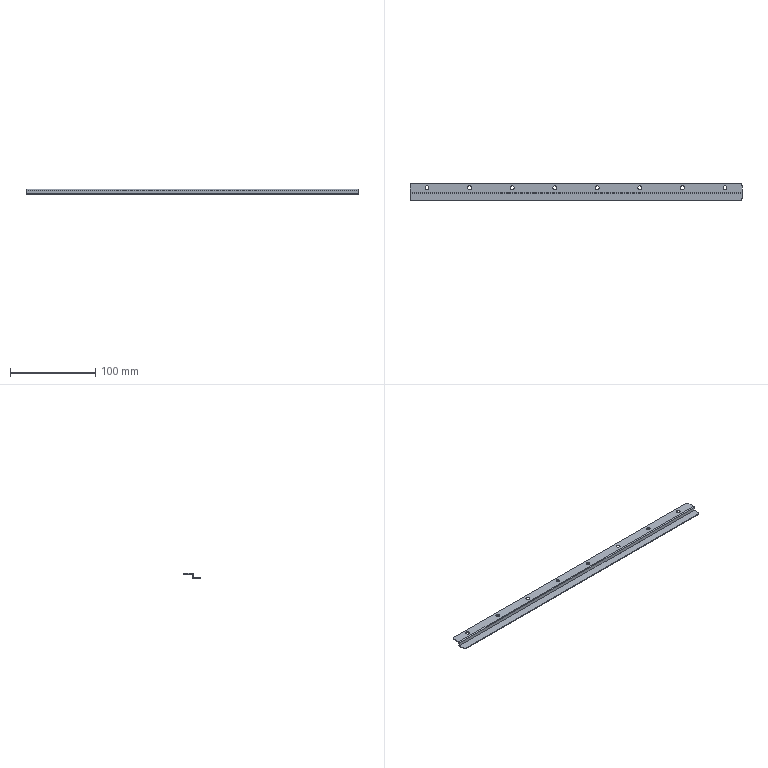Part | STEP file | 1 solid | 42 faces | box 390 x 21 x 6 mm | volume 9834 mm3 | cylinder 24 | plane 18 | commonest cylinder face diameters 4.5 x16 6 x4 0.02 x2 2.02 x2